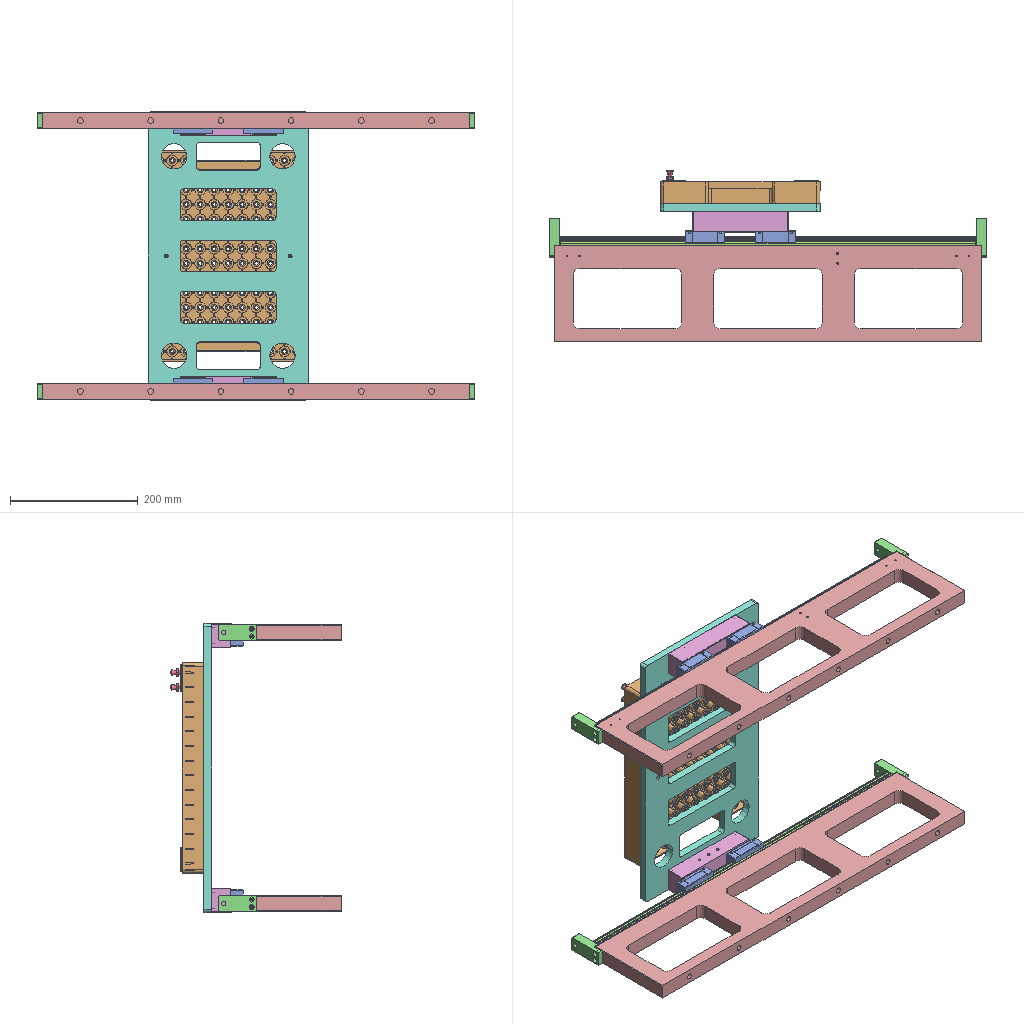Assembly | SolidWorks | 10 different items | 22 placed | box 686 x 269 x 453 mm
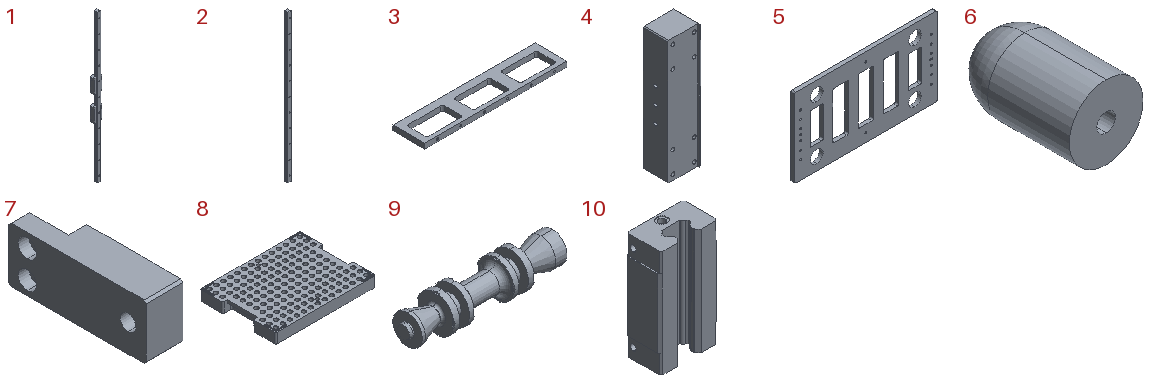Parts list (item | name | quantity | parent item | size | volume | features):
1 | (subassembly) | x2 | - | 34 x 24 x 650 mm | 182322 mm3 | -
2 | - | x2 | in 1 | 15 x 15 x 650 mm | 119721 mm3 | features MoveFace 2, BaseBody 1, LPattern 1
3 | - | x2 | - | 670 x 150 x 24 mm | 1244825 mm3 | features HoleWzd 7, Chamfer 1, Extrusion 1, ICE 1
4 | - | x2 | - | 38 x 32 x 150 mm | 164701 mm3 | features HoleWzd 4, Chamfer 1, Extrusion 1
5 | - | x1 | - | 453 x 12 x 250 mm | 916603 mm3 | features HoleWzd 5, Fillet 3, ICE 2, Extrusion 1
6 | - | x2 | - | 9.95 x 15.5 x 9.95 mm | 1091 mm3 | features HoleWzd 1, Revolution 1
7 | - | x4 | - | 16 x 60 x 24 mm | 18592 mm3 | features BaseBody 1, Chamfer 1, HoleWzd 1, ICE 1
8 | - | x1 | - | - | 715592 mm3 | features BaseBody 1
9 | - | x2 | - | 49.9 x 12 x 12 mm | 2556 mm3 | features Fillet 2, Chamfer 1, CirPattern 1, ICE 1, MirrorPattern 1, Revolution 1
10 | - | x4 | in 1 | 34 x 19.7 x 61.4 mm | 31300 mm3 | features BaseBody 1
Mates (type | each side: item.copy, entity, surface, feature):
In the top assembly
Coincident | 3.1 face plane Boss-Extrude1 | 2.1 face plane Input1
Concentric | 3.1 face cylinder M4 Tapped Hole1 | 2.1 face cylinder Input1
Parallel | 3.1 face plane Boss-Extrude1 | 2.1 face plane Input1
Concentric | 2.2 face cylinder Input1 | 3.2 face cylinder M4 Tapped Hole1
Coincident | 2.2 face plane Input1 | 3.2 face plane Boss-Extrude1
Parallel | 2.2 face plane Input1 | 3.2 face plane Boss-Extrude1
Coincident | 3.1 face plane Boss-Extrude1 | 3.2 face plane Boss-Extrude1 | 2 times
DistanceDim | 3.2 face plane Boss-Extrude1 | 3.1 face plane Boss-Extrude1
Coincident | 10.1 face plane Input1 | 4.1 face plane Boss-Extrude1 | 3 times
Coincident | 10.2 face plane Input1 | 4.2 face plane Boss-Extrude1 | 3 times
Coincident | 10.1 face plane Input1 | 10.3 face plane Input1
Coincident | 4.2 face plane Boss-Extrude1 | 5.1 face plane Boss-Extrude1
Width | 5.1 face plane Boss-Extrude1 | 5.1 face plane Boss-Extrude1 | 4.1 face plane Boss-Extrude1 | 4.1 face plane Boss-Extrude1
Width | 5.1 face plane Boss-Extrude1 | 5.1 face plane Boss-Extrude1 | 4.2 face plane Boss-Extrude1 | 4.1 face plane Boss-Extrude1
Concentric | 5.1 face cylinder Cut-Extrude1 | 8.1 face cylinder Input1 | 2 times
Coincident | 5.1 face plane Boss-Extrude1 | 8.1 face plane Input1
Concentric | 5.1 face cylinder Cut-Extrude1 | 6.1 face cylinder Revolve1
Coincident | 5.1 face plane Cut-Extrude1 | 6.1 face plane Revolve1
Coincident | 5.1 face plane Cut-Extrude1 | 6.2 face plane Revolve1
Concentric | 5.1 face cylinder Cut-Extrude1 | 6.2 face cylinder Revolve1
Coincident | 3.2 face plane Boss-Extrude1 | 7.1 face plane Input1
Concentric | 3.2 face cylinder M4 Tapped Hole3 | 7.1 face cylinder Input1 | 2 times
Coincident | 3.2 face plane Boss-Extrude1 | 7.2 face plane Input1
Concentric | 3.2 face cylinder M4 Tapped Hole2 | 7.2 face cylinder Input1 | 2 times
Coincident | 3.1 face plane Boss-Extrude1 | 7.3 face plane Input1
Concentric | 3.1 face cylinder M4 Tapped Hole3 | 7.3 face cylinder Input1 | 2 times
Coincident | 3.1 face plane Boss-Extrude1 | 7.4 face plane Input1
Concentric | 3.1 face cylinder M4 Tapped Hole2 | 7.4 face cylinder Input1 | 2 times
Coincident | 8.1 face plane Input1 | 9.1 face plane Revolve1
Concentric | 8.1 face cone Input1 | 9.1 face cylinder Revolve1
Coincident | 8.1 face plane Input1 | 9.2 face plane Revolve1
Concentric | 8.1 face cone Input1 | 9.2 face cylinder Revolve1
In subassembly 1
Coincident | 10.4 face plane Input1 | 2.3 face plane Input1
Width | 10.4 face plane Input1 | 10.4 face plane Input1 | 2.3 face plane Input1 | 2.3 face plane Input1
Coincident | 2.3 face plane Input1 | 10.5 face plane Input1
Width | 10.5 face plane Input1 | 10.5 face plane Input1 | 2.3 face plane Input1 | 2.3 face plane Input1
LimitDistanceDim | 10.4 face plane Input1 | 2.3 face plane Input1
LimitDistanceDim | 10.5 face plane Input1 | 2.3 face plane Input1
DistanceDim | 10.4 face plane Input1 | 10.5 face plane Input1